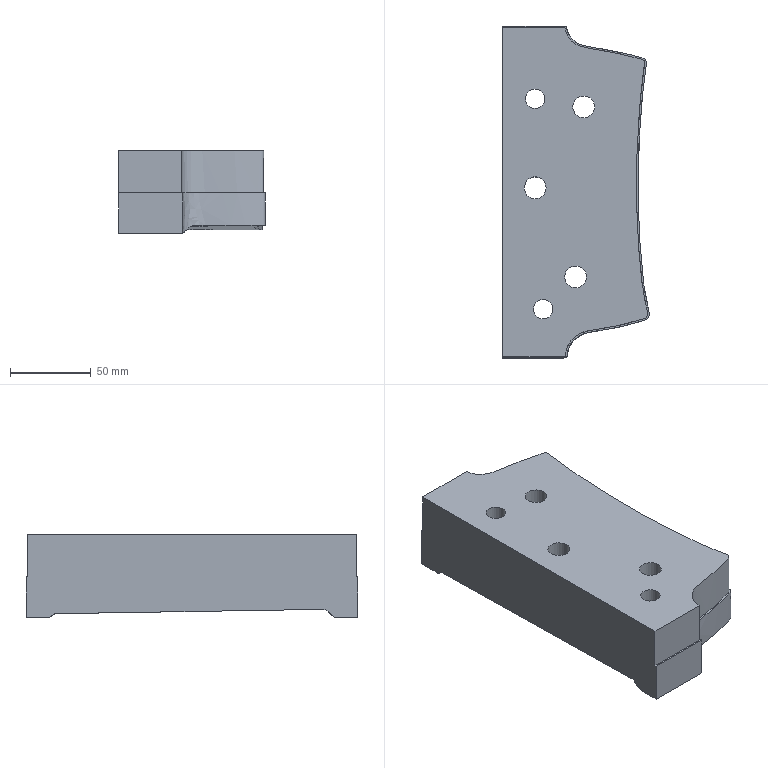Part | NX | features solid 2 | 1 solid | 43 faces | box 90.456 x 205 x 51 mm | volume 693482 mm3 | plane 17 | cylinder 15 | spline 9 | sphere 2 | commonest cylinder face diameters 10 x3 13.5 x3 19.5 x3 6 x2 12 x2 13 x2